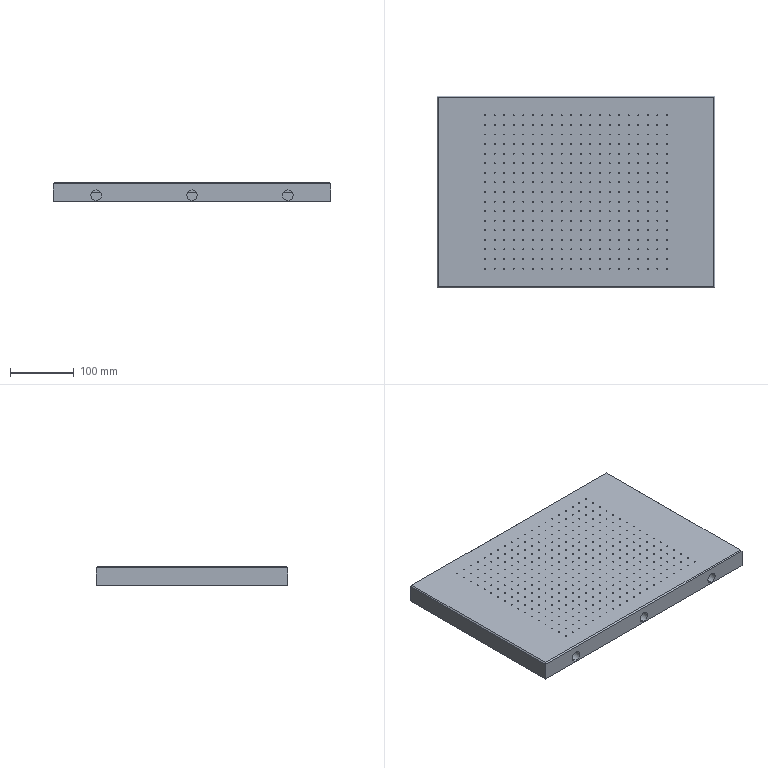Part | STEP file | Platform 1 (default) | 1 solid | 727 faces | box 435 x 300 x 30 mm | volume 1924051 mm3 | cylinder 686 | plane 41 | commonest cylinder face diameters 1.5 x680 16.5 x6